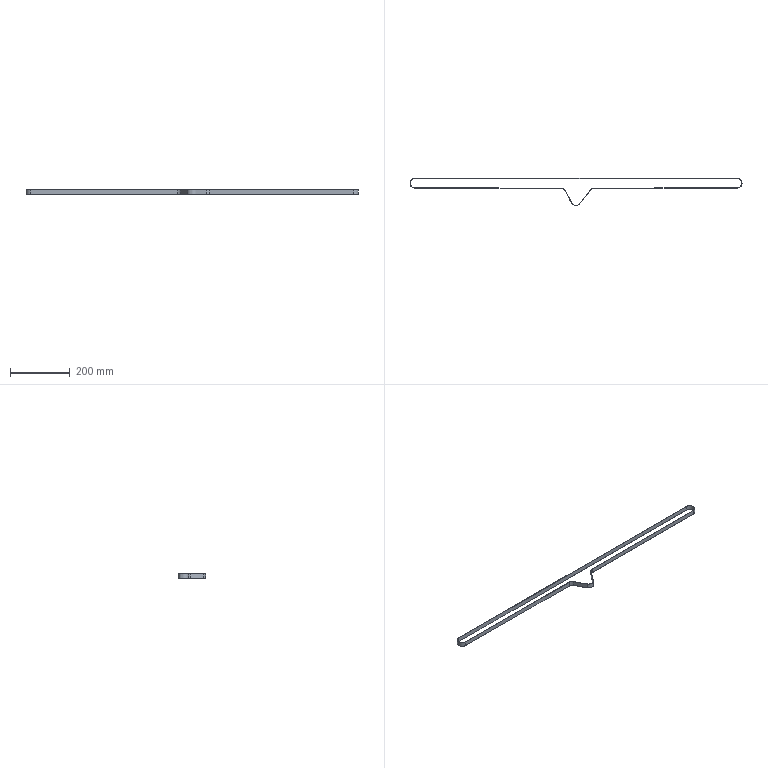Part | NX | 1 solid | 22 faces | box 1113 x 92 x 15 mm | volume 34767 mm3 | plane 12 | cylinder 10 | commonest cylinder face diameters 31 x5 33 x3 29 x2
STEP:
#1=CARTESIAN_POINT('',(401.038,-31.78,7.5));
#2=VERTEX_POINT('',#1);
#3=CARTESIAN_POINT('',(428.591,-33.971,7.5));
#4=VERTEX_POINT('',#3);
#5=CARTESIAN_POINT('',(415.529,-23.89,7.5));
#6=DIRECTION('',(0.,0.,1.));
#7=DIRECTION('',(1.,0.,0.));
#8=AXIS2_PLACEMENT_3D('',#5,#6,#7);
#9=CIRCLE('',#8,16.5);
#10=EDGE_CURVE('',#2,#4,#9,.T.);
#11=ORIENTED_EDGE('',*,*,#10,.T.);
#12=CARTESIAN_POINT('',(464.051,11.97,7.5));
#13=VERTEX_POINT('',#12);
#14=CARTESIAN_POINT('',(428.591,-33.971,7.5));
#15=DIRECTION('',(0.611,0.7916,0.));
#16=VECTOR('',#15,1000.);
#17=LINE('',#14,#16);
#18=EDGE_CURVE('',#4,#13,#17,.T.);
#19=ORIENTED_EDGE('',*,*,#18,.T.);
#20=CARTESIAN_POINT('',(475.499,17.61,7.5));
#21=VERTEX_POINT('',#20);
#22=CARTESIAN_POINT('',(475.529,3.11,7.5));
#23=DIRECTION('',(0.,0.,1.));
#24=DIRECTION('',(1.,0.,0.));
#25=AXIS2_PLACEMENT_3D('',#22,#23,#24);
#26=CIRCLE('',#25,14.5);
#27=EDGE_CURVE('',#13,#21,#26,.F.);
#28=ORIENTED_EDGE('',*,*,#27,.T.);
#29=CARTESIAN_POINT('',(955.563,18.611,7.5));
#30=VERTEX_POINT('',#29);
#31=CARTESIAN_POINT('',(475.499,17.61,7.5));
#32=DIRECTION('',(1.,0.002083,0.));
#33=VECTOR('',#32,1000.);
#34=LINE('',#31,#33);
#35=EDGE_CURVE('',#21,#30,#34,.T.);
#36=ORIENTED_EDGE('',*,*,#35,.T.);
#37=CARTESIAN_POINT('',(955.529,51.61,7.5));
#38=VERTEX_POINT('',#37);
#39=CARTESIAN_POINT('',(955.546,35.111,7.5));
#40=DIRECTION('',(0.,0.,1.));
#41=DIRECTION('',(1.,0.,0.));
#42=AXIS2_PLACEMENT_3D('',#39,#40,#41);
#43=CIRCLE('',#42,16.5);
#44=EDGE_CURVE('',#30,#38,#43,.T.);
#45=ORIENTED_EDGE('',*,*,#44,.T.);
#46=CARTESIAN_POINT('',(-124.471,51.61,7.5));
#47=VERTEX_POINT('',#46);
#48=CARTESIAN_POINT('',(955.529,51.61,7.5));
#49=DIRECTION('',(-1.,0.,0.));
#50=VECTOR('',#49,1000.);
#51=LINE('',#48,#50);
#52=EDGE_CURVE('',#38,#47,#51,.T.);
#53=ORIENTED_EDGE('',*,*,#52,.T.);
#54=CARTESIAN_POINT('',(-124.504,18.611,7.5));
#55=VERTEX_POINT('',#54);
#56=CARTESIAN_POINT('',(-124.471,35.11,7.5));
#57=DIRECTION('',(0.,0.,1.));
#58=DIRECTION('',(1.,0.,0.));
#59=AXIS2_PLACEMENT_3D('',#56,#57,#58);
#60=CIRCLE('',#59,16.5);
#61=EDGE_CURVE('',#47,#55,#60,.T.);
#62=ORIENTED_EDGE('',*,*,#61,.T.);
#63=CARTESIAN_POINT('',(365.559,17.61,7.5));
#64=VERTEX_POINT('',#63);
#65=CARTESIAN_POINT('',(-124.504,18.611,7.5));
#66=DIRECTION('',(1.,-0.002041,0.));
#67=VECTOR('',#66,1000.);
#68=LINE('',#65,#67);
#69=EDGE_CURVE('',#55,#64,#68,.T.);
#70=ORIENTED_EDGE('',*,*,#69,.T.);
#71=CARTESIAN_POINT('',(378.264,10.045,7.5));
#72=VERTEX_POINT('',#71);
#73=CARTESIAN_POINT('',(365.529,3.11,7.5));
#74=DIRECTION('',(0.,0.,1.));
#75=DIRECTION('',(1.,0.,0.));
#76=AXIS2_PLACEMENT_3D('',#73,#74,#75);
#77=CIRCLE('',#76,14.5);
#78=EDGE_CURVE('',#64,#72,#77,.F.);
#79=ORIENTED_EDGE('',*,*,#78,.T.);
#80=CARTESIAN_POINT('',(378.264,10.045,7.5));
#81=DIRECTION('',(0.4782,-0.8782,0.));
#82=VECTOR('',#81,1000.);
#83=LINE('',#80,#82);
#84=EDGE_CURVE('',#72,#2,#83,.T.);
#85=ORIENTED_EDGE('',*,*,#84,.T.);
#86=EDGE_LOOP('',(#11,#19,#28,#36,#45,#53,#62,#70,#79,#85));
#87=FACE_BOUND('',#86,.T.);
#88=CARTESIAN_POINT('',(427.8,-33.36,7.5));
#89=VERTEX_POINT('',#88);
#90=CARTESIAN_POINT('',(463.259,12.581,7.5));
#91=VERTEX_POINT('',#90);
#92=CARTESIAN_POINT('',(427.8,-33.36,7.5));
#93=DIRECTION('',(0.611,0.7916,0.));
#94=VECTOR('',#93,1000.);
#95=LINE('',#92,#94);
#96=EDGE_CURVE('',#89,#91,#95,.T.);
#97=ORIENTED_EDGE('',*,*,#96,.F.);
#98=CARTESIAN_POINT('',(401.917,-31.302,7.5));
#99=VERTEX_POINT('',#98);
#100=CARTESIAN_POINT('',(415.529,-23.89,7.5));
#101=DIRECTION('',(0.,0.,1.));
#102=DIRECTION('',(1.,0.,0.));
#103=AXIS2_PLACEMENT_3D('',#100,#101,#102);
#104=CIRCLE('',#103,15.5);
#105=EDGE_CURVE('',#99,#89,#104,.T.);
#106=ORIENTED_EDGE('',*,*,#105,.F.);
#107=CARTESIAN_POINT('',(379.142,10.523,7.5));
#108=VERTEX_POINT('',#107);
#109=CARTESIAN_POINT('',(379.142,10.523,7.5));
#110=DIRECTION('',(0.4782,-0.8782,0.));
#111=VECTOR('',#110,1000.);
#112=LINE('',#109,#111);
#113=EDGE_CURVE('',#108,#99,#112,.T.);
#114=ORIENTED_EDGE('',*,*,#113,.F.);
#115=CARTESIAN_POINT('',(365.561,18.61,7.5));
#116=VERTEX_POINT('',#115);
#117=CARTESIAN_POINT('',(365.529,3.11,7.5));
#118=DIRECTION('',(0.,0.,-1.));
#119=DIRECTION('',(-1.,0.,0.));
#120=AXIS2_PLACEMENT_3D('',#117,#118,#119);
#121=CIRCLE('',#120,15.5);
#122=EDGE_CURVE('',#116,#108,#121,.T.);
#123=ORIENTED_EDGE('',*,*,#122,.F.);
#124=CARTESIAN_POINT('',(-124.502,19.611,7.5));
#125=VERTEX_POINT('',#124);
#126=CARTESIAN_POINT('',(-124.502,19.611,7.5));
#127=DIRECTION('',(1.,-0.002041,0.));
#128=VECTOR('',#127,1000.);
#129=LINE('',#126,#128);
#130=EDGE_CURVE('',#125,#116,#129,.T.);
#131=ORIENTED_EDGE('',*,*,#130,.F.);
#132=CARTESIAN_POINT('',(-124.471,50.61,7.5));
#133=VERTEX_POINT('',#132);
#134=CARTESIAN_POINT('',(-124.471,35.11,7.5));
#135=DIRECTION('',(0.,0.,1.));
#136=DIRECTION('',(1.,0.,0.));
#137=AXIS2_PLACEMENT_3D('',#134,#135,#136);
#138=CIRCLE('',#137,15.5);
#139=EDGE_CURVE('',#133,#125,#138,.T.);
#140=ORIENTED_EDGE('',*,*,#139,.F.);
#141=CARTESIAN_POINT('',(955.529,50.61,7.5));
#142=VERTEX_POINT('',#141);
#143=CARTESIAN_POINT('',(955.529,50.61,7.5));
#144=DIRECTION('',(-1.,0.,0.));
#145=VECTOR('',#144,1000.);
#146=LINE('',#143,#145);
#147=EDGE_CURVE('',#142,#133,#146,.T.);
#148=ORIENTED_EDGE('',*,*,#147,.F.);
#149=CARTESIAN_POINT('',(955.562,19.611,7.5));
#150=VERTEX_POINT('',#149);
#151=CARTESIAN_POINT('',(955.546,35.111,7.5));
#152=DIRECTION('',(0.,0.,1.));
#153=DIRECTION('',(1.,0.,0.));
#154=AXIS2_PLACEMENT_3D('',#151,#152,#153);
#155=CIRCLE('',#154,15.5);
#156=EDGE_CURVE('',#150,#142,#155,.T.);
#157=ORIENTED_EDGE('',*,*,#156,.F.);
#158=CARTESIAN_POINT('',(475.497,18.61,7.5));
#159=VERTEX_POINT('',#158);
#160=CARTESIAN_POINT('',(475.497,18.61,7.5));
#161=DIRECTION('',(1.,0.002083,0.));
#162=VECTOR('',#161,1000.);
#163=LINE('',#160,#162);
#164=EDGE_CURVE('',#159,#150,#163,.T.);
#165=ORIENTED_EDGE('',*,*,#164,.F.);
#166=CARTESIAN_POINT('',(475.529,3.11,7.5));
#167=DIRECTION('',(0.,0.,-1.));
#168=DIRECTION('',(-1.,0.,0.));
#169=AXIS2_PLACEMENT_3D('',#166,#167,#168);
#170=CIRCLE('',#169,15.5);
#171=EDGE_CURVE('',#91,#159,#170,.T.);
#172=ORIENTED_EDGE('',*,*,#171,.F.);
#173=EDGE_LOOP('',(#97,#106,#114,#123,#131,#140,#148,#157,#165,#172));
#174=FACE_BOUND('',#173,.T.);
#175=CARTESIAN_POINT('',(415.529,-23.89,7.5));
#176=DIRECTION('',(0.,0.,1.));
#177=DIRECTION('',(1.,0.,0.));
#178=AXIS2_PLACEMENT_3D('',#175,#176,#177);
#179=PLANE('',#178);
#180=ADVANCED_FACE('',(#87,#174),#179,.T.);
#181=CARTESIAN_POINT('',(401.038,-31.78,-7.5));
#182=VERTEX_POINT('',#181);
#183=CARTESIAN_POINT('',(428.591,-33.971,-7.5));
#184=VERTEX_POINT('',#183);
#185=CARTESIAN_POINT('',(415.529,-23.89,-7.5));
#186=DIRECTION('',(0.,0.,1.));
#187=DIRECTION('',(1.,0.,0.));
#188=AXIS2_PLACEMENT_3D('',#185,#186,#187);
#189=CIRCLE('',#188,16.5);
#190=EDGE_CURVE('',#182,#184,#189,.T.);
#191=ORIENTED_EDGE('',*,*,#190,.F.);
#192=CARTESIAN_POINT('',(378.264,10.045,-7.5));
#193=VERTEX_POINT('',#192);
#194=CARTESIAN_POINT('',(378.264,10.045,-7.5));
#195=DIRECTION('',(0.4782,-0.8782,0.));
#196=VECTOR('',#195,1000.);
#197=LINE('',#194,#196);
#198=EDGE_CURVE('',#193,#182,#197,.T.);
#199=ORIENTED_EDGE('',*,*,#198,.F.);
#200=CARTESIAN_POINT('',(365.559,17.61,-7.5));
#201=VERTEX_POINT('',#200);
#202=CARTESIAN_POINT('',(365.529,3.11,-7.5));
#203=DIRECTION('',(0.,0.,1.));
#204=DIRECTION('',(1.,0.,0.));
#205=AXIS2_PLACEMENT_3D('',#202,#203,#204);
#206=CIRCLE('',#205,14.5);
#207=EDGE_CURVE('',#201,#193,#206,.F.);
#208=ORIENTED_EDGE('',*,*,#207,.F.);
#209=CARTESIAN_POINT('',(-124.504,18.611,-7.5));
#210=VERTEX_POINT('',#209);
#211=CARTESIAN_POINT('',(-124.504,18.611,-7.5));
#212=DIRECTION('',(1.,-0.002041,0.));
#213=VECTOR('',#212,1000.);
#214=LINE('',#211,#213);
#215=EDGE_CURVE('',#210,#201,#214,.T.);
#216=ORIENTED_EDGE('',*,*,#215,.F.);
#217=CARTESIAN_POINT('',(-124.471,51.61,-7.5));
#218=VERTEX_POINT('',#217);
#219=CARTESIAN_POINT('',(-124.471,35.11,-7.5));
#220=DIRECTION('',(0.,0.,1.));
#221=DIRECTION('',(1.,0.,0.));
#222=AXIS2_PLACEMENT_3D('',#219,#220,#221);
#223=CIRCLE('',#222,16.5);
#224=EDGE_CURVE('',#218,#210,#223,.T.);
#225=ORIENTED_EDGE('',*,*,#224,.F.);
#226=CARTESIAN_POINT('',(955.529,51.61,-7.5));
#227=VERTEX_POINT('',#226);
#228=CARTESIAN_POINT('',(955.529,51.61,-7.5));
#229=DIRECTION('',(-1.,0.,0.));
#230=VECTOR('',#229,1000.);
#231=LINE('',#228,#230);
#232=EDGE_CURVE('',#227,#218,#231,.T.);
#233=ORIENTED_EDGE('',*,*,#232,.F.);
#234=CARTESIAN_POINT('',(955.563,18.611,-7.5));
#235=VERTEX_POINT('',#234);
#236=CARTESIAN_POINT('',(955.546,35.111,-7.5));
#237=DIRECTION('',(0.,0.,1.));
#238=DIRECTION('',(1.,0.,0.));
#239=AXIS2_PLACEMENT_3D('',#236,#237,#238);
#240=CIRCLE('',#239,16.5);
#241=EDGE_CURVE('',#235,#227,#240,.T.);
#242=ORIENTED_EDGE('',*,*,#241,.F.);
#243=CARTESIAN_POINT('',(475.499,17.61,-7.5));
#244=VERTEX_POINT('',#243);
#245=CARTESIAN_POINT('',(475.499,17.61,-7.5));
#246=DIRECTION('',(1.,0.002083,0.));
#247=VECTOR('',#246,1000.);
#248=LINE('',#245,#247);
#249=EDGE_CURVE('',#244,#235,#248,.T.);
#250=ORIENTED_EDGE('',*,*,#249,.F.);
#251=CARTESIAN_POINT('',(464.051,11.97,-7.5));
#252=VERTEX_POINT('',#251);
#253=CARTESIAN_POINT('',(475.529,3.11,-7.5));
#254=DIRECTION('',(0.,0.,1.));
#255=DIRECTION('',(1.,0.,0.));
#256=AXIS2_PLACEMENT_3D('',#253,#254,#255);
#257=CIRCLE('',#256,14.5);
#258=EDGE_CURVE('',#252,#244,#257,.F.);
#259=ORIENTED_EDGE('',*,*,#258,.F.);
#260=CARTESIAN_POINT('',(428.591,-33.971,-7.5));
#261=DIRECTION('',(0.611,0.7916,0.));
#262=VECTOR('',#261,1000.);
#263=LINE('',#260,#262);
#264=EDGE_CURVE('',#184,#252,#263,.T.);
#265=ORIENTED_EDGE('',*,*,#264,.F.);
#266=EDGE_LOOP('',(#191,#199,#208,#216,#225,#233,#242,#250,#259,#265));
#267=FACE_BOUND('',#266,.T.);
#268=CARTESIAN_POINT('',(401.917,-31.302,-7.5));
#269=VERTEX_POINT('',#268);
#270=CARTESIAN_POINT('',(427.8,-33.36,-7.5));
#271=VERTEX_POINT('',#270);
#272=CARTESIAN_POINT('',(415.529,-23.89,-7.5));
#273=DIRECTION('',(0.,0.,1.));
#274=DIRECTION('',(1.,0.,0.));
#275=AXIS2_PLACEMENT_3D('',#272,#273,#274);
#276=CIRCLE('',#275,15.5);
#277=EDGE_CURVE('',#269,#271,#276,.T.);
#278=ORIENTED_EDGE('',*,*,#277,.T.);
#279=CARTESIAN_POINT('',(463.259,12.581,-7.5));
#280=VERTEX_POINT('',#279);
#281=CARTESIAN_POINT('',(427.8,-33.36,-7.5));
#282=DIRECTION('',(0.611,0.7916,0.));
#283=VECTOR('',#282,1000.);
#284=LINE('',#281,#283);
#285=EDGE_CURVE('',#271,#280,#284,.T.);
#286=ORIENTED_EDGE('',*,*,#285,.T.);
#287=CARTESIAN_POINT('',(475.497,18.61,-7.5));
#288=VERTEX_POINT('',#287);
#289=CARTESIAN_POINT('',(475.529,3.11,-7.5));
#290=DIRECTION('',(0.,0.,-1.));
#291=DIRECTION('',(-1.,0.,0.));
#292=AXIS2_PLACEMENT_3D('',#289,#290,#291);
#293=CIRCLE('',#292,15.5);
#294=EDGE_CURVE('',#280,#288,#293,.T.);
#295=ORIENTED_EDGE('',*,*,#294,.T.);
#296=CARTESIAN_POINT('',(955.562,19.611,-7.5));
#297=VERTEX_POINT('',#296);
#298=CARTESIAN_POINT('',(475.497,18.61,-7.5));
#299=DIRECTION('',(1.,0.002083,0.));
#300=VECTOR('',#299,1000.);
#301=LINE('',#298,#300);
#302=EDGE_CURVE('',#288,#297,#301,.T.);
#303=ORIENTED_EDGE('',*,*,#302,.T.);
#304=CARTESIAN_POINT('',(955.529,50.61,-7.5));
#305=VERTEX_POINT('',#304);
#306=CARTESIAN_POINT('',(955.546,35.111,-7.5));
#307=DIRECTION('',(0.,0.,1.));
#308=DIRECTION('',(1.,0.,0.));
#309=AXIS2_PLACEMENT_3D('',#306,#307,#308);
#310=CIRCLE('',#309,15.5);
#311=EDGE_CURVE('',#297,#305,#310,.T.);
#312=ORIENTED_EDGE('',*,*,#311,.T.);
#313=CARTESIAN_POINT('',(-124.471,50.61,-7.5));
#314=VERTEX_POINT('',#313);
#315=CARTESIAN_POINT('',(955.529,50.61,-7.5));
#316=DIRECTION('',(-1.,0.,0.));
#317=VECTOR('',#316,1000.);
#318=LINE('',#315,#317);
#319=EDGE_CURVE('',#305,#314,#318,.T.);
#320=ORIENTED_EDGE('',*,*,#319,.T.);
#321=CARTESIAN_POINT('',(-124.502,19.611,-7.5));
#322=VERTEX_POINT('',#321);
#323=CARTESIAN_POINT('',(-124.471,35.11,-7.5));
#324=DIRECTION('',(0.,0.,1.));
#325=DIRECTION('',(1.,0.,0.));
#326=AXIS2_PLACEMENT_3D('',#323,#324,#325);
#327=CIRCLE('',#326,15.5);
#328=EDGE_CURVE('',#314,#322,#327,.T.);
#329=ORIENTED_EDGE('',*,*,#328,.T.);
#330=CARTESIAN_POINT('',(365.561,18.61,-7.5));
#331=VERTEX_POINT('',#330);
#332=CARTESIAN_POINT('',(-124.502,19.611,-7.5));
#333=DIRECTION('',(1.,-0.002041,0.));
#334=VECTOR('',#333,1000.);
#335=LINE('',#332,#334);
#336=EDGE_CURVE('',#322,#331,#335,.T.);
#337=ORIENTED_EDGE('',*,*,#336,.T.);
#338=CARTESIAN_POINT('',(379.142,10.523,-7.5));
#339=VERTEX_POINT('',#338);
#340=CARTESIAN_POINT('',(365.529,3.11,-7.5));
#341=DIRECTION('',(0.,0.,-1.));
#342=DIRECTION('',(-1.,0.,0.));
#343=AXIS2_PLACEMENT_3D('',#340,#341,#342);
#344=CIRCLE('',#343,15.5);
#345=EDGE_CURVE('',#331,#339,#344,.T.);
#346=ORIENTED_EDGE('',*,*,#345,.T.);
#347=CARTESIAN_POINT('',(379.142,10.523,-7.5));
#348=DIRECTION('',(0.4782,-0.8782,0.));
#349=VECTOR('',#348,1000.);
#350=LINE('',#347,#349);
#351=EDGE_CURVE('',#339,#269,#350,.T.);
#352=ORIENTED_EDGE('',*,*,#351,.T.);
#353=EDGE_LOOP('',(#278,#286,#295,#303,#312,#320,#329,#337,#346,#352));
#354=FACE_BOUND('',#353,.T.);
#355=CARTESIAN_POINT('',(415.529,-23.89,-7.5));
#356=DIRECTION('',(0.,0.,1.));
#357=DIRECTION('',(1.,0.,0.));
#358=AXIS2_PLACEMENT_3D('',#355,#356,#357);
#359=PLANE('',#358);
#360=ADVANCED_FACE('',(#267,#354),#359,.F.);
#361=ORIENTED_EDGE('',*,*,#190,.T.);
#362=CARTESIAN_POINT('',(428.591,-33.971,7.5));
#363=DIRECTION('',(0.,0.,-1.));
#364=VECTOR('',#363,1000.);
#365=LINE('',#362,#364);
#366=EDGE_CURVE('',#4,#184,#365,.T.);
#367=ORIENTED_EDGE('',*,*,#366,.F.);
#368=ORIENTED_EDGE('',*,*,#10,.F.);
#369=CARTESIAN_POINT('',(401.038,-31.78,7.5));
#370=DIRECTION('',(0.,0.,-1.));
#371=VECTOR('',#370,1000.);
#372=LINE('',#369,#371);
#373=EDGE_CURVE('',#2,#182,#372,.T.);
#374=ORIENTED_EDGE('',*,*,#373,.T.);
#375=EDGE_LOOP('',(#361,#367,#368,#374));
#376=FACE_BOUND('',#375,.T.);
#377=CARTESIAN_POINT('',(415.529,-23.89,7.5));
#378=DIRECTION('',(0.,0.,-1.));
#379=DIRECTION('',(-1.,0.,0.));
#380=AXIS2_PLACEMENT_3D('',#377,#378,#379);
#381=CYLINDRICAL_SURFACE('',#380,16.5);
#382=ADVANCED_FACE('',(#376),#381,.T.);
#383=ORIENTED_EDGE('',*,*,#264,.T.);
#384=CARTESIAN_POINT('',(464.051,11.97,7.5));
#385=DIRECTION('',(0.,0.,-1.));
#386=VECTOR('',#385,1000.);
#387=LINE('',#384,#386);
#388=EDGE_CURVE('',#13,#252,#387,.T.);
#389=ORIENTED_EDGE('',*,*,#388,.F.);
#390=ORIENTED_EDGE('',*,*,#18,.F.);
#391=ORIENTED_EDGE('',*,*,#366,.T.);
#392=EDGE_LOOP('',(#383,#389,#390,#391));
#393=FACE_BOUND('',#392,.T.);
#394=CARTESIAN_POINT('',(428.591,-33.971,7.5));
#395=DIRECTION('',(-0.7916,0.611,0.));
#396=DIRECTION('',(-0.611,-0.7916,0.));
#397=AXIS2_PLACEMENT_3D('',#394,#395,#396);
#398=PLANE('',#397);
#399=ADVANCED_FACE('',(#393),#398,.F.);
#400=ORIENTED_EDGE('',*,*,#258,.T.);
#401=CARTESIAN_POINT('',(475.499,17.61,7.5));
#402=DIRECTION('',(0.,0.,-1.));
#403=VECTOR('',#402,1000.);
#404=LINE('',#401,#403);
#405=EDGE_CURVE('',#21,#244,#404,.T.);
#406=ORIENTED_EDGE('',*,*,#405,.F.);
#407=ORIENTED_EDGE('',*,*,#27,.F.);
#408=ORIENTED_EDGE('',*,*,#388,.T.);
#409=EDGE_LOOP('',(#400,#406,#407,#408));
#410=FACE_BOUND('',#409,.T.);
#411=CARTESIAN_POINT('',(475.529,3.11,7.5));
#412=DIRECTION('',(0.,0.,-1.));
#413=DIRECTION('',(-1.,0.,0.));
#414=AXIS2_PLACEMENT_3D('',#411,#412,#413);
#415=CYLINDRICAL_SURFACE('',#414,14.5);
#416=ADVANCED_FACE('',(#410),#415,.F.);
#417=ORIENTED_EDGE('',*,*,#249,.T.);
#418=CARTESIAN_POINT('',(955.563,18.611,7.5));
#419=DIRECTION('',(0.,0.,-1.));
#420=VECTOR('',#419,1000.);
#421=LINE('',#418,#420);
#422=EDGE_CURVE('',#30,#235,#421,.T.);
#423=ORIENTED_EDGE('',*,*,#422,.F.);
#424=ORIENTED_EDGE('',*,*,#35,.F.);
#425=ORIENTED_EDGE('',*,*,#405,.T.);
#426=EDGE_LOOP('',(#417,#423,#424,#425));
#427=FACE_BOUND('',#426,.T.);
#428=CARTESIAN_POINT('',(475.499,17.61,7.5));
#429=DIRECTION('',(-0.002083,1.,0.));
#430=DIRECTION('',(-1.,-0.002083,0.));
#431=AXIS2_PLACEMENT_3D('',#428,#429,#430);
#432=PLANE('',#431);
#433=ADVANCED_FACE('',(#427),#432,.F.);
#434=ORIENTED_EDGE('',*,*,#241,.T.);
#435=CARTESIAN_POINT('',(955.529,51.61,7.5));
#436=DIRECTION('',(0.,0.,-1.));
#437=VECTOR('',#436,1000.);
#438=LINE('',#435,#437);
#439=EDGE_CURVE('',#38,#227,#438,.T.);
#440=ORIENTED_EDGE('',*,*,#439,.F.);
#441=ORIENTED_EDGE('',*,*,#44,.F.);
#442=ORIENTED_EDGE('',*,*,#422,.T.);
#443=EDGE_LOOP('',(#434,#440,#441,#442));
#444=FACE_BOUND('',#443,.T.);
#445=CARTESIAN_POINT('',(955.546,35.111,7.5));
#446=DIRECTION('',(0.,0.,-1.));
#447=DIRECTION('',(-1.,0.,0.));
#448=AXIS2_PLACEMENT_3D('',#445,#446,#447);
#449=CYLINDRICAL_SURFACE('',#448,16.5);
#450=ADVANCED_FACE('',(#444),#449,.T.);
#451=ORIENTED_EDGE('',*,*,#232,.T.);
#452=CARTESIAN_POINT('',(-124.471,51.61,7.5));
#453=DIRECTION('',(0.,0.,-1.));
#454=VECTOR('',#453,1000.);
#455=LINE('',#452,#454);
#456=EDGE_CURVE('',#47,#218,#455,.T.);
#457=ORIENTED_EDGE('',*,*,#456,.F.);
#458=ORIENTED_EDGE('',*,*,#52,.F.);
#459=ORIENTED_EDGE('',*,*,#439,.T.);
#460=EDGE_LOOP('',(#451,#457,#458,#459));
#461=FACE_BOUND('',#460,.T.);
#462=CARTESIAN_POINT('',(955.529,51.61,7.5));
#463=DIRECTION('',(0.,-1.,0.));
#464=DIRECTION('',(0.,0.,-1.));
#465=AXIS2_PLACEMENT_3D('',#462,#463,#464);
#466=PLANE('',#465);
#467=ADVANCED_FACE('',(#461),#466,.F.);
#468=ORIENTED_EDGE('',*,*,#224,.T.);
#469=CARTESIAN_POINT('',(-124.504,18.611,7.5));
#470=DIRECTION('',(0.,0.,-1.));
#471=VECTOR('',#470,1000.);
#472=LINE('',#469,#471);
#473=EDGE_CURVE('',#55,#210,#472,.T.);
#474=ORIENTED_EDGE('',*,*,#473,.F.);
#475=ORIENTED_EDGE('',*,*,#61,.F.);
#476=ORIENTED_EDGE('',*,*,#456,.T.);
#477=EDGE_LOOP('',(#468,#474,#475,#476));
#478=FACE_BOUND('',#477,.T.);
#479=CARTESIAN_POINT('',(-124.471,35.11,7.5));
#480=DIRECTION('',(0.,0.,-1.));
#481=DIRECTION('',(-1.,0.,0.));
#482=AXIS2_PLACEMENT_3D('',#479,#480,#481);
#483=CYLINDRICAL_SURFACE('',#482,16.5);
#484=ADVANCED_FACE('',(#478),#483,.T.);
#485=ORIENTED_EDGE('',*,*,#215,.T.);
#486=CARTESIAN_POINT('',(365.559,17.61,7.5));
#487=DIRECTION('',(0.,0.,-1.));
#488=VECTOR('',#487,1000.);
#489=LINE('',#486,#488);
#490=EDGE_CURVE('',#64,#201,#489,.T.);
#491=ORIENTED_EDGE('',*,*,#490,.F.);
#492=ORIENTED_EDGE('',*,*,#69,.F.);
#493=ORIENTED_EDGE('',*,*,#473,.T.);
#494=EDGE_LOOP('',(#485,#491,#492,#493));
#495=FACE_BOUND('',#494,.T.);
#496=CARTESIAN_POINT('',(-124.504,18.611,7.5));
#497=DIRECTION('',(0.002041,1.,0.));
#498=DIRECTION('',(-1.,0.002041,0.));
#499=AXIS2_PLACEMENT_3D('',#496,#497,#498);
#500=PLANE('',#499);
#501=ADVANCED_FACE('',(#495),#500,.F.);
#502=ORIENTED_EDGE('',*,*,#207,.T.);
#503=CARTESIAN_POINT('',(378.264,10.045,7.5));
#504=DIRECTION('',(0.,0.,-1.));
#505=VECTOR('',#504,1000.);
#506=LINE('',#503,#505);
#507=EDGE_CURVE('',#72,#193,#506,.T.);
#508=ORIENTED_EDGE('',*,*,#507,.F.);
#509=ORIENTED_EDGE('',*,*,#78,.F.);
#510=ORIENTED_EDGE('',*,*,#490,.T.);
#511=EDGE_LOOP('',(#502,#508,#509,#510));
#512=FACE_BOUND('',#511,.T.);
#513=CARTESIAN_POINT('',(365.529,3.11,7.5));
#514=DIRECTION('',(0.,0.,-1.));
#515=DIRECTION('',(-1.,0.,0.));
#516=AXIS2_PLACEMENT_3D('',#513,#514,#515);
#517=CYLINDRICAL_SURFACE('',#516,14.5);
#518=ADVANCED_FACE('',(#512),#517,.F.);
#519=ORIENTED_EDGE('',*,*,#198,.T.);
#520=ORIENTED_EDGE('',*,*,#373,.F.);
#521=ORIENTED_EDGE('',*,*,#84,.F.);
#522=ORIENTED_EDGE('',*,*,#507,.T.);
#523=EDGE_LOOP('',(#519,#520,#521,#522));
#524=FACE_BOUND('',#523,.T.);
#525=CARTESIAN_POINT('',(378.264,10.045,7.5));
#526=DIRECTION('',(0.8782,0.4782,0.));
#527=DIRECTION('',(-0.4782,0.8782,0.));
#528=AXIS2_PLACEMENT_3D('',#525,#526,#527);
#529=PLANE('',#528);
#530=ADVANCED_FACE('',(#524),#529,.F.);
#531=ORIENTED_EDGE('',*,*,#277,.F.);
#532=CARTESIAN_POINT('',(401.917,-31.302,7.5));
#533=DIRECTION('',(0.,0.,-1.));
#534=VECTOR('',#533,1000.);
#535=LINE('',#532,#534);
#536=EDGE_CURVE('',#99,#269,#535,.T.);
#537=ORIENTED_EDGE('',*,*,#536,.F.);
#538=ORIENTED_EDGE('',*,*,#105,.T.);
#539=CARTESIAN_POINT('',(427.8,-33.36,7.5));
#540=DIRECTION('',(0.,0.,-1.));
#541=VECTOR('',#540,1000.);
#542=LINE('',#539,#541);
#543=EDGE_CURVE('',#89,#271,#542,.T.);
#544=ORIENTED_EDGE('',*,*,#543,.T.);
#545=EDGE_LOOP('',(#531,#537,#538,#544));
#546=FACE_BOUND('',#545,.T.);
#547=CARTESIAN_POINT('',(415.529,-23.89,7.5));
#548=DIRECTION('',(0.,0.,-1.));
#549=DIRECTION('',(-1.,0.,0.));
#550=AXIS2_PLACEMENT_3D('',#547,#548,#549);
#551=CYLINDRICAL_SURFACE('',#550,15.5);
#552=ADVANCED_FACE('',(#546),#551,.F.);
#553=ORIENTED_EDGE('',*,*,#285,.F.);
#554=ORIENTED_EDGE('',*,*,#543,.F.);
#555=ORIENTED_EDGE('',*,*,#96,.T.);
#556=CARTESIAN_POINT('',(463.259,12.581,7.5));
#557=DIRECTION('',(0.,0.,-1.));
#558=VECTOR('',#557,1000.);
#559=LINE('',#556,#558);
#560=EDGE_CURVE('',#91,#280,#559,.T.);
#561=ORIENTED_EDGE('',*,*,#560,.T.);
#562=EDGE_LOOP('',(#553,#554,#555,#561));
#563=FACE_BOUND('',#562,.T.);
#564=CARTESIAN_POINT('',(427.8,-33.36,7.5));
#565=DIRECTION('',(-0.7916,0.611,0.));
#566=DIRECTION('',(-0.611,-0.7916,0.));
#567=AXIS2_PLACEMENT_3D('',#564,#565,#566);
#568=PLANE('',#567);
#569=ADVANCED_FACE('',(#563),#568,.T.);
#570=ORIENTED_EDGE('',*,*,#294,.F.);
#571=ORIENTED_EDGE('',*,*,#560,.F.);
#572=ORIENTED_EDGE('',*,*,#171,.T.);
#573=CARTESIAN_POINT('',(475.497,18.61,7.5));
#574=DIRECTION('',(0.,0.,-1.));
#575=VECTOR('',#574,1000.);
#576=LINE('',#573,#575);
#577=EDGE_CURVE('',#159,#288,#576,.T.);
#578=ORIENTED_EDGE('',*,*,#577,.T.);
#579=EDGE_LOOP('',(#570,#571,#572,#578));
#580=FACE_BOUND('',#579,.T.);
#581=CARTESIAN_POINT('',(475.529,3.11,7.5));
#582=DIRECTION('',(0.,0.,-1.));
#583=DIRECTION('',(-1.,0.,0.));
#584=AXIS2_PLACEMENT_3D('',#581,#582,#583);
#585=CYLINDRICAL_SURFACE('',#584,15.5);
#586=ADVANCED_FACE('',(#580),#585,.T.);
#587=ORIENTED_EDGE('',*,*,#302,.F.);
#588=ORIENTED_EDGE('',*,*,#577,.F.);
#589=ORIENTED_EDGE('',*,*,#164,.T.);
#590=CARTESIAN_POINT('',(955.562,19.611,7.5));
#591=DIRECTION('',(0.,0.,-1.));
#592=VECTOR('',#591,1000.);
#593=LINE('',#590,#592);
#594=EDGE_CURVE('',#150,#297,#593,.T.);
#595=ORIENTED_EDGE('',*,*,#594,.T.);
#596=EDGE_LOOP('',(#587,#588,#589,#595));
#597=FACE_BOUND('',#596,.T.);
#598=CARTESIAN_POINT('',(475.497,18.61,7.5));
#599=DIRECTION('',(-0.002083,1.,0.));
#600=DIRECTION('',(-1.,-0.002083,0.));
#601=AXIS2_PLACEMENT_3D('',#598,#599,#600);
#602=PLANE('',#601);
#603=ADVANCED_FACE('',(#597),#602,.T.);
#604=ORIENTED_EDGE('',*,*,#311,.F.);
#605=ORIENTED_EDGE('',*,*,#594,.F.);
#606=ORIENTED_EDGE('',*,*,#156,.T.);
#607=CARTESIAN_POINT('',(955.529,50.61,7.5));
#608=DIRECTION('',(0.,0.,-1.));
#609=VECTOR('',#608,1000.);
#610=LINE('',#607,#609);
#611=EDGE_CURVE('',#142,#305,#610,.T.);
#612=ORIENTED_EDGE('',*,*,#611,.T.);
#613=EDGE_LOOP('',(#604,#605,#606,#612));
#614=FACE_BOUND('',#613,.T.);
#615=CARTESIAN_POINT('',(955.546,35.111,7.5));
#616=DIRECTION('',(0.,0.,-1.));
#617=DIRECTION('',(-1.,0.,0.));
#618=AXIS2_PLACEMENT_3D('',#615,#616,#617);
#619=CYLINDRICAL_SURFACE('',#618,15.5);
#620=ADVANCED_FACE('',(#614),#619,.F.);
#621=ORIENTED_EDGE('',*,*,#319,.F.);
#622=ORIENTED_EDGE('',*,*,#611,.F.);
#623=ORIENTED_EDGE('',*,*,#147,.T.);
#624=CARTESIAN_POINT('',(-124.471,50.61,7.5));
#625=DIRECTION('',(0.,0.,-1.));
#626=VECTOR('',#625,1000.);
#627=LINE('',#624,#626);
#628=EDGE_CURVE('',#133,#314,#627,.T.);
#629=ORIENTED_EDGE('',*,*,#628,.T.);
#630=EDGE_LOOP('',(#621,#622,#623,#629));
#631=FACE_BOUND('',#630,.T.);
#632=CARTESIAN_POINT('',(955.529,50.61,7.5));
#633=DIRECTION('',(0.,-1.,0.));
#634=DIRECTION('',(0.,0.,-1.));
#635=AXIS2_PLACEMENT_3D('',#632,#633,#634);
#636=PLANE('',#635);
#637=ADVANCED_FACE('',(#631),#636,.T.);
#638=ORIENTED_EDGE('',*,*,#328,.F.);
#639=ORIENTED_EDGE('',*,*,#628,.F.);
#640=ORIENTED_EDGE('',*,*,#139,.T.);
#641=CARTESIAN_POINT('',(-124.502,19.611,7.5));
#642=DIRECTION('',(0.,0.,-1.));
#643=VECTOR('',#642,1000.);
#644=LINE('',#641,#643);
#645=EDGE_CURVE('',#125,#322,#644,.T.);
#646=ORIENTED_EDGE('',*,*,#645,.T.);
#647=EDGE_LOOP('',(#638,#639,#640,#646));
#648=FACE_BOUND('',#647,.T.);
#649=CARTESIAN_POINT('',(-124.471,35.11,7.5));
#650=DIRECTION('',(0.,0.,-1.));
#651=DIRECTION('',(-1.,0.,0.));
#652=AXIS2_PLACEMENT_3D('',#649,#650,#651);
#653=CYLINDRICAL_SURFACE('',#652,15.5);
#654=ADVANCED_FACE('',(#648),#653,.F.);
#655=ORIENTED_EDGE('',*,*,#336,.F.);
#656=ORIENTED_EDGE('',*,*,#645,.F.);
#657=ORIENTED_EDGE('',*,*,#130,.T.);
#658=CARTESIAN_POINT('',(365.561,18.61,7.5));
#659=DIRECTION('',(0.,0.,-1.));
#660=VECTOR('',#659,1000.);
#661=LINE('',#658,#660);
#662=EDGE_CURVE('',#116,#331,#661,.T.);
#663=ORIENTED_EDGE('',*,*,#662,.T.);
#664=EDGE_LOOP('',(#655,#656,#657,#663));
#665=FACE_BOUND('',#664,.T.);
#666=CARTESIAN_POINT('',(-124.502,19.611,7.5));
#667=DIRECTION('',(0.002041,1.,0.));
#668=DIRECTION('',(-1.,0.002041,0.));
#669=AXIS2_PLACEMENT_3D('',#666,#667,#668);
#670=PLANE('',#669);
#671=ADVANCED_FACE('',(#665),#670,.T.);
#672=ORIENTED_EDGE('',*,*,#345,.F.);
#673=ORIENTED_EDGE('',*,*,#662,.F.);
#674=ORIENTED_EDGE('',*,*,#122,.T.);
#675=CARTESIAN_POINT('',(379.142,10.523,7.5));
#676=DIRECTION('',(0.,0.,-1.));
#677=VECTOR('',#676,1000.);
#678=LINE('',#675,#677);
#679=EDGE_CURVE('',#108,#339,#678,.T.);
#680=ORIENTED_EDGE('',*,*,#679,.T.);
#681=EDGE_LOOP('',(#672,#673,#674,#680));
#682=FACE_BOUND('',#681,.T.);
#683=CARTESIAN_POINT('',(365.529,3.11,7.5));
#684=DIRECTION('',(0.,0.,-1.));
#685=DIRECTION('',(-1.,0.,0.));
#686=AXIS2_PLACEMENT_3D('',#683,#684,#685);
#687=CYLINDRICAL_SURFACE('',#686,15.5);
#688=ADVANCED_FACE('',(#682),#687,.T.);
#689=ORIENTED_EDGE('',*,*,#351,.F.);
#690=ORIENTED_EDGE('',*,*,#679,.F.);
#691=ORIENTED_EDGE('',*,*,#113,.T.);
#692=ORIENTED_EDGE('',*,*,#536,.T.);
#693=EDGE_LOOP('',(#689,#690,#691,#692));
#694=FACE_BOUND('',#693,.T.);
#695=CARTESIAN_POINT('',(379.142,10.523,7.5));
#696=DIRECTION('',(0.8782,0.4782,0.));
#697=DIRECTION('',(-0.4782,0.8782,0.));
#698=AXIS2_PLACEMENT_3D('',#695,#696,#697);
#699=PLANE('',#698);
#700=ADVANCED_FACE('',(#694),#699,.T.);
#701=CLOSED_SHELL('',(#180,#360,#382,#399,#416,#433,#450,#467,#484,#501,#518,#530,#552,#569,#586,#603,#620,#637,#654,#671,#688,#700));
#702=MANIFOLD_SOLID_BREP('',#701);
#703=(LENGTH_UNIT()NAMED_UNIT(*)SI_UNIT(.MILLI.,.METRE.));
#704=UNCERTAINTY_MEASURE_WITH_UNIT(LENGTH_MEASURE(0.00001),#703,'','');
#705=(NAMED_UNIT(*)PLANE_ANGLE_UNIT()SI_UNIT($,.RADIAN.));
#706=(NAMED_UNIT(*)SI_UNIT($,.STERADIAN.)SOLID_ANGLE_UNIT());
#707=(GEOMETRIC_REPRESENTATION_CONTEXT(3)GLOBAL_UNCERTAINTY_ASSIGNED_CONTEXT((#704))GLOBAL_UNIT_ASSIGNED_CONTEXT((#703,#705,#706))REPRESENTATION_CONTEXT('',''));
#708=ADVANCED_BREP_SHAPE_REPRESENTATION('',(#702),#707);